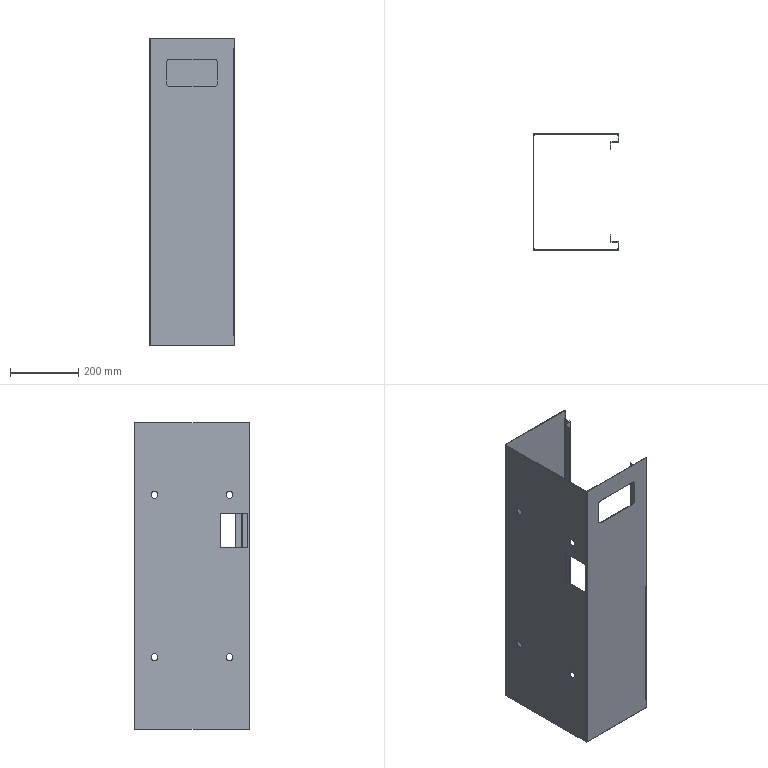Part | SolidWorks | features EdgeFlange 6, Cut 3, FlatPattern 1, LPattern 1, SMBaseFlange 1, SheetMetal 1 | 1 solid | 106 faces | box 250 x 340 x 900 mm | volume 1255343 mm3 | plane 78 | cylinder 28 | commonest cylinder face diameters 20 x12 2 x8 5 x8